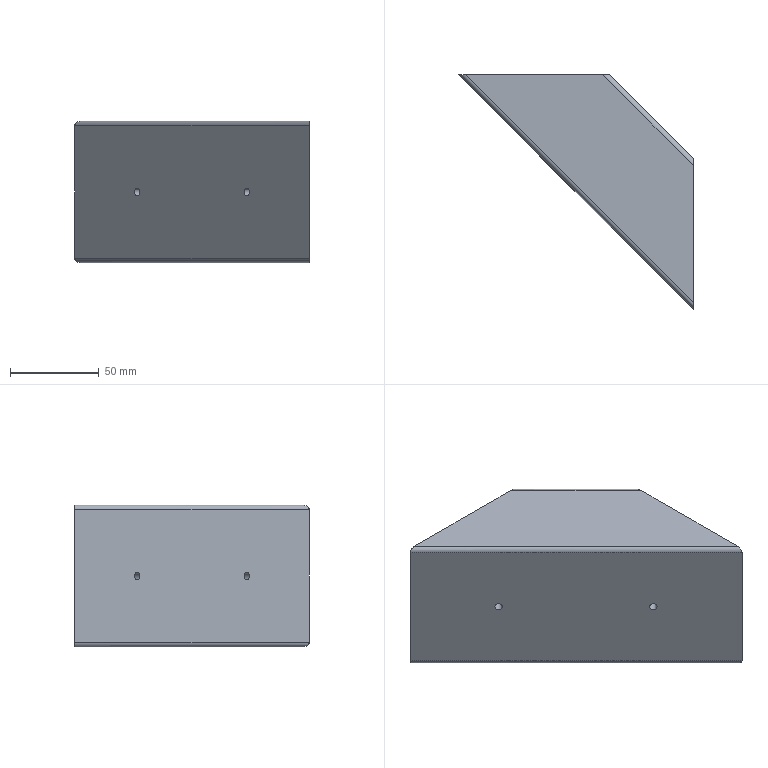Part | NX | 1 solid | 20 faces | box 132.426 x 132.426 x 80 mm | volume 195335 mm3 | plane 10 | cylinder 10 | commonest cylinder face diameters 5.236 x8 4.2 x2
STEP:
#1=CARTESIAN_POINT('',(-86.059,505.,-31.382));
#2=VERTEX_POINT('',#1);
#3=CARTESIAN_POINT('',(-89.761,505.,-34.));
#4=VERTEX_POINT('',#3);
#5=CARTESIAN_POINT('',(-89.761,505.,-31.382));
#6=DIRECTION('',(0.,1.,0.));
#7=DIRECTION('',(-1.,0.,0.));
#8=AXIS2_PLACEMENT_3D('',#5,#6,#7);
#9=ELLIPSE('',#8,3.702,2.618);
#10=EDGE_CURVE('',#2,#4,#9,.T.);
#11=ORIENTED_EDGE('',*,*,#10,.F.);
#12=CARTESIAN_POINT('',(-86.059,505.,31.382));
#13=VERTEX_POINT('',#12);
#14=CARTESIAN_POINT('',(-86.059,505.,31.382));
#15=DIRECTION('',(0.,0.,-1.));
#16=VECTOR('',#15,1000.);
#17=LINE('',#14,#16);
#18=EDGE_CURVE('',#13,#2,#17,.T.);
#19=ORIENTED_EDGE('',*,*,#18,.F.);
#20=CARTESIAN_POINT('',(-89.761,505.,34.));
#21=VERTEX_POINT('',#20);
#22=CARTESIAN_POINT('',(-89.761,505.,31.382));
#23=DIRECTION('',(0.,1.,0.));
#24=DIRECTION('',(-1.,0.,0.));
#25=AXIS2_PLACEMENT_3D('',#22,#23,#24);
#26=ELLIPSE('',#25,3.702,2.618);
#27=EDGE_CURVE('',#21,#13,#26,.T.);
#28=ORIENTED_EDGE('',*,*,#27,.F.);
#29=CARTESIAN_POINT('',(-150.239,505.,34.));
#30=VERTEX_POINT('',#29);
#31=CARTESIAN_POINT('',(-15.119,505.,34.));
#32=DIRECTION('',(1.,0.,0.));
#33=VECTOR('',#32,1000.);
#34=LINE('',#31,#33);
#35=EDGE_CURVE('',#30,#21,#34,.T.);
#36=ORIENTED_EDGE('',*,*,#35,.F.);
#37=CARTESIAN_POINT('',(-153.941,505.,31.382));
#38=VERTEX_POINT('',#37);
#39=CARTESIAN_POINT('',(-150.239,505.,31.382));
#40=DIRECTION('',(0.,1.,0.));
#41=DIRECTION('',(-1.,0.,0.));
#42=AXIS2_PLACEMENT_3D('',#39,#40,#41);
#43=ELLIPSE('',#42,3.702,2.618);
#44=EDGE_CURVE('',#38,#30,#43,.T.);
#45=ORIENTED_EDGE('',*,*,#44,.F.);
#46=CARTESIAN_POINT('',(-153.941,505.,-31.382));
#47=VERTEX_POINT('',#46);
#48=CARTESIAN_POINT('',(-153.941,505.,31.382));
#49=DIRECTION('',(0.,0.,1.));
#50=VECTOR('',#49,1000.);
#51=LINE('',#48,#50);
#52=EDGE_CURVE('',#47,#38,#51,.T.);
#53=ORIENTED_EDGE('',*,*,#52,.F.);
#54=CARTESIAN_POINT('',(-150.239,505.,-34.));
#55=VERTEX_POINT('',#54);
#56=CARTESIAN_POINT('',(-150.239,505.,-31.382));
#57=DIRECTION('',(0.,1.,0.));
#58=DIRECTION('',(-1.,0.,0.));
#59=AXIS2_PLACEMENT_3D('',#56,#57,#58);
#60=ELLIPSE('',#59,3.702,2.618);
#61=EDGE_CURVE('',#55,#47,#60,.T.);
#62=ORIENTED_EDGE('',*,*,#61,.F.);
#63=CARTESIAN_POINT('',(-15.119,505.,-34.));
#64=DIRECTION('',(-1.,0.,0.));
#65=VECTOR('',#64,1000.);
#66=LINE('',#63,#65);
#67=EDGE_CURVE('',#4,#55,#66,.T.);
#68=ORIENTED_EDGE('',*,*,#67,.F.);
#69=EDGE_LOOP('',(#11,#19,#28,#36,#45,#53,#62,#68));
#70=FACE_BOUND('',#69,.T.);
#71=CARTESIAN_POINT('',(-158.724,505.,-40.));
#72=VERTEX_POINT('',#71);
#73=CARTESIAN_POINT('',(-162.426,505.,-37.382));
#74=VERTEX_POINT('',#73);
#75=CARTESIAN_POINT('',(-158.724,505.,-37.382));
#76=DIRECTION('',(0.,1.,0.));
#77=DIRECTION('',(-1.,0.,0.));
#78=AXIS2_PLACEMENT_3D('',#75,#76,#77);
#79=ELLIPSE('',#78,3.702,2.618);
#80=EDGE_CURVE('',#72,#74,#79,.T.);
#81=ORIENTED_EDGE('',*,*,#80,.T.);
#82=CARTESIAN_POINT('',(-162.426,505.,37.382));
#83=VERTEX_POINT('',#82);
#84=CARTESIAN_POINT('',(-162.426,505.,37.382));
#85=DIRECTION('',(0.,0.,1.));
#86=VECTOR('',#85,1000.);
#87=LINE('',#84,#86);
#88=EDGE_CURVE('',#74,#83,#87,.T.);
#89=ORIENTED_EDGE('',*,*,#88,.T.);
#90=CARTESIAN_POINT('',(-158.724,505.,40.));
#91=VERTEX_POINT('',#90);
#92=CARTESIAN_POINT('',(-158.724,505.,37.382));
#93=DIRECTION('',(0.,1.,0.));
#94=DIRECTION('',(-1.,0.,0.));
#95=AXIS2_PLACEMENT_3D('',#92,#93,#94);
#96=ELLIPSE('',#95,3.702,2.618);
#97=EDGE_CURVE('',#83,#91,#96,.T.);
#98=ORIENTED_EDGE('',*,*,#97,.T.);
#99=CARTESIAN_POINT('',(-81.276,505.,40.));
#100=VERTEX_POINT('',#99);
#101=CARTESIAN_POINT('',(1126.,505.,40.));
#102=DIRECTION('',(-1.,0.,0.));
#103=VECTOR('',#102,1000.);
#104=LINE('',#101,#103);
#105=EDGE_CURVE('',#100,#91,#104,.T.);
#106=ORIENTED_EDGE('',*,*,#105,.F.);
#107=CARTESIAN_POINT('',(-77.574,505.,37.382));
#108=VERTEX_POINT('',#107);
#109=CARTESIAN_POINT('',(-81.276,505.,37.382));
#110=DIRECTION('',(0.,1.,0.));
#111=DIRECTION('',(-1.,0.,0.));
#112=AXIS2_PLACEMENT_3D('',#109,#110,#111);
#113=ELLIPSE('',#112,3.702,2.618);
#114=EDGE_CURVE('',#100,#108,#113,.T.);
#115=ORIENTED_EDGE('',*,*,#114,.T.);
#116=CARTESIAN_POINT('',(-77.574,505.,-37.382));
#117=VERTEX_POINT('',#116);
#118=CARTESIAN_POINT('',(-77.574,505.,37.382));
#119=DIRECTION('',(0.,0.,-1.));
#120=VECTOR('',#119,1000.);
#121=LINE('',#118,#120);
#122=EDGE_CURVE('',#108,#117,#121,.T.);
#123=ORIENTED_EDGE('',*,*,#122,.T.);
#124=CARTESIAN_POINT('',(-81.276,505.,-40.));
#125=VERTEX_POINT('',#124);
#126=CARTESIAN_POINT('',(-81.276,505.,-37.382));
#127=DIRECTION('',(0.,1.,0.));
#128=DIRECTION('',(-1.,0.,0.));
#129=AXIS2_PLACEMENT_3D('',#126,#127,#128);
#130=ELLIPSE('',#129,3.702,2.618);
#131=EDGE_CURVE('',#117,#125,#130,.T.);
#132=ORIENTED_EDGE('',*,*,#131,.T.);
#133=CARTESIAN_POINT('',(1126.,505.,-40.));
#134=DIRECTION('',(-1.,0.,0.));
#135=VECTOR('',#134,1000.);
#136=LINE('',#133,#135);
#137=EDGE_CURVE('',#125,#72,#136,.T.);
#138=ORIENTED_EDGE('',*,*,#137,.T.);
#139=EDGE_LOOP('',(#81,#89,#98,#106,#115,#123,#132,#138));
#140=FACE_BOUND('',#139,.T.);
#141=CARTESIAN_POINT('',(1126.,505.,37.382));
#142=DIRECTION('',(0.,1.,0.));
#143=DIRECTION('',(0.,0.,1.));
#144=AXIS2_PLACEMENT_3D('',#141,#142,#143);
#145=PLANE('',#144);
#146=ADVANCED_FACE('',(#70,#140),#145,.T.);
#147=ORIENTED_EDGE('',*,*,#114,.F.);
#148=CARTESIAN_POINT('',(-30.,453.724,40.));
#149=VERTEX_POINT('',#148);
#150=CARTESIAN_POINT('',(19.362,404.362,40.));
#151=DIRECTION('',(-0.7071,0.7071,0.));
#152=VECTOR('',#151,1000.);
#153=LINE('',#150,#152);
#154=EDGE_CURVE('',#149,#100,#153,.T.);
#155=ORIENTED_EDGE('',*,*,#154,.F.);
#156=CARTESIAN_POINT('',(-30.,457.426,37.382));
#157=VERTEX_POINT('',#156);
#158=CARTESIAN_POINT('',(-30.,453.724,37.382));
#159=DIRECTION('',(1.,0.,0.));
#160=DIRECTION('',(0.,1.,0.));
#161=AXIS2_PLACEMENT_3D('',#158,#159,#160);
#162=ELLIPSE('',#161,3.702,2.618);
#163=EDGE_CURVE('',#157,#149,#162,.T.);
#164=ORIENTED_EDGE('',*,*,#163,.F.);
#165=CARTESIAN_POINT('',(21.213,406.213,37.382));
#166=DIRECTION('',(-0.7071,0.7071,0.));
#167=VECTOR('',#166,1000.);
#168=LINE('',#165,#167);
#169=EDGE_CURVE('',#157,#108,#168,.T.);
#170=ORIENTED_EDGE('',*,*,#169,.T.);
#171=EDGE_LOOP('',(#147,#155,#164,#170));
#172=FACE_BOUND('',#171,.T.);
#173=CARTESIAN_POINT('',(19.362,404.362,37.382));
#174=DIRECTION('',(-0.7071,0.7071,0.));
#175=DIRECTION('',(-0.7071,-0.7071,0.));
#176=AXIS2_PLACEMENT_3D('',#173,#174,#175);
#177=CYLINDRICAL_SURFACE('',#176,2.618);
#178=ADVANCED_FACE('',(#172),#177,.T.);
#179=ORIENTED_EDGE('',*,*,#105,.T.);
#180=CARTESIAN_POINT('',(-30.,376.276,40.));
#181=VERTEX_POINT('',#180);
#182=CARTESIAN_POINT('',(-19.362,365.638,40.));
#183=DIRECTION('',(-0.7071,0.7071,0.));
#184=VECTOR('',#183,1000.);
#185=LINE('',#182,#184);
#186=EDGE_CURVE('',#181,#91,#185,.T.);
#187=ORIENTED_EDGE('',*,*,#186,.F.);
#188=CARTESIAN_POINT('',(-30.,535.,40.));
#189=DIRECTION('',(0.,-1.,0.));
#190=VECTOR('',#189,1000.);
#191=LINE('',#188,#190);
#192=EDGE_CURVE('',#149,#181,#191,.T.);
#193=ORIENTED_EDGE('',*,*,#192,.F.);
#194=ORIENTED_EDGE('',*,*,#154,.T.);
#195=EDGE_LOOP('',(#179,#187,#193,#194));
#196=FACE_BOUND('',#195,.T.);
#197=CARTESIAN_POINT('',(-19.362,365.638,40.));
#198=DIRECTION('',(0.,0.,-1.));
#199=DIRECTION('',(-1.,0.,0.));
#200=AXIS2_PLACEMENT_3D('',#197,#198,#199);
#201=PLANE('',#200);
#202=ADVANCED_FACE('',(#196),#201,.F.);
#203=ORIENTED_EDGE('',*,*,#97,.F.);
#204=CARTESIAN_POINT('',(-30.,372.574,37.382));
#205=VERTEX_POINT('',#204);
#206=CARTESIAN_POINT('',(-21.213,363.787,37.382));
#207=DIRECTION('',(-0.7071,0.7071,0.));
#208=VECTOR('',#207,1000.);
#209=LINE('',#206,#208);
#210=EDGE_CURVE('',#205,#83,#209,.T.);
#211=ORIENTED_EDGE('',*,*,#210,.F.);
#212=CARTESIAN_POINT('',(-30.,376.276,37.382));
#213=DIRECTION('',(1.,0.,0.));
#214=DIRECTION('',(0.,1.,0.));
#215=AXIS2_PLACEMENT_3D('',#212,#213,#214);
#216=ELLIPSE('',#215,3.702,2.618);
#217=EDGE_CURVE('',#181,#205,#216,.T.);
#218=ORIENTED_EDGE('',*,*,#217,.F.);
#219=ORIENTED_EDGE('',*,*,#186,.T.);
#220=EDGE_LOOP('',(#203,#211,#218,#219));
#221=FACE_BOUND('',#220,.T.);
#222=CARTESIAN_POINT('',(-19.362,365.638,37.382));
#223=DIRECTION('',(-0.7071,0.7071,0.));
#224=DIRECTION('',(-0.7071,-0.7071,0.));
#225=AXIS2_PLACEMENT_3D('',#222,#223,#224);
#226=CYLINDRICAL_SURFACE('',#225,2.618);
#227=ADVANCED_FACE('',(#221),#226,.T.);
#228=CARTESIAN_POINT('',(-66.84,409.414,0.));
#229=VERTEX_POINT('',#228);
#230=CARTESIAN_POINT('',(-65.355,407.929,0.));
#231=DIRECTION('',(-0.7071,-0.7071,0.));
#232=DIRECTION('',(-0.7071,0.7071,0.));
#233=AXIS2_PLACEMENT_3D('',#230,#231,#232);
#234=CIRCLE('',#233,2.1);
#235=EDGE_CURVE('',#229,#229,#234,.T.);
#236=ORIENTED_EDGE('',*,*,#235,.F.);
#237=EDGE_LOOP('',(#236));
#238=FACE_BOUND('',#237,.T.);
#239=CARTESIAN_POINT('',(-128.556,471.13,0.));
#240=VERTEX_POINT('',#239);
#241=CARTESIAN_POINT('',(-127.071,469.645,0.));
#242=DIRECTION('',(-0.7071,-0.7071,0.));
#243=DIRECTION('',(-0.7071,0.7071,0.));
#244=AXIS2_PLACEMENT_3D('',#241,#242,#243);
#245=CIRCLE('',#244,2.1);
#246=EDGE_CURVE('',#240,#240,#245,.T.);
#247=ORIENTED_EDGE('',*,*,#246,.F.);
#248=EDGE_LOOP('',(#247));
#249=FACE_BOUND('',#248,.T.);
#250=ORIENTED_EDGE('',*,*,#88,.F.);
#251=CARTESIAN_POINT('',(-30.,372.574,-37.382));
#252=VERTEX_POINT('',#251);
#253=CARTESIAN_POINT('',(-21.213,363.787,-37.382));
#254=DIRECTION('',(-0.7071,0.7071,0.));
#255=VECTOR('',#254,1000.);
#256=LINE('',#253,#255);
#257=EDGE_CURVE('',#252,#74,#256,.T.);
#258=ORIENTED_EDGE('',*,*,#257,.F.);
#259=CARTESIAN_POINT('',(-30.,372.574,37.382));
#260=DIRECTION('',(0.,0.,-1.));
#261=VECTOR('',#260,1000.);
#262=LINE('',#259,#261);
#263=EDGE_CURVE('',#205,#252,#262,.T.);
#264=ORIENTED_EDGE('',*,*,#263,.F.);
#265=ORIENTED_EDGE('',*,*,#210,.T.);
#266=EDGE_LOOP('',(#250,#258,#264,#265));
#267=FACE_BOUND('',#266,.T.);
#268=CARTESIAN_POINT('',(-21.213,363.787,37.382));
#269=DIRECTION('',(0.7071,0.7071,0.));
#270=DIRECTION('',(-0.7071,0.7071,0.));
#271=AXIS2_PLACEMENT_3D('',#268,#269,#270);
#272=PLANE('',#271);
#273=ADVANCED_FACE('',(#238,#249,#267),#272,.F.);
#274=ORIENTED_EDGE('',*,*,#80,.F.);
#275=CARTESIAN_POINT('',(-30.,376.276,-40.));
#276=VERTEX_POINT('',#275);
#277=CARTESIAN_POINT('',(-19.362,365.638,-40.));
#278=DIRECTION('',(-0.7071,0.7071,0.));
#279=VECTOR('',#278,1000.);
#280=LINE('',#277,#279);
#281=EDGE_CURVE('',#276,#72,#280,.T.);
#282=ORIENTED_EDGE('',*,*,#281,.F.);
#283=CARTESIAN_POINT('',(-30.,376.276,-37.382));
#284=DIRECTION('',(1.,0.,0.));
#285=DIRECTION('',(0.,1.,0.));
#286=AXIS2_PLACEMENT_3D('',#283,#284,#285);
#287=ELLIPSE('',#286,3.702,2.618);
#288=EDGE_CURVE('',#252,#276,#287,.T.);
#289=ORIENTED_EDGE('',*,*,#288,.F.);
#290=ORIENTED_EDGE('',*,*,#257,.T.);
#291=EDGE_LOOP('',(#274,#282,#289,#290));
#292=FACE_BOUND('',#291,.T.);
#293=CARTESIAN_POINT('',(-19.362,365.638,-37.382));
#294=DIRECTION('',(-0.7071,0.7071,0.));
#295=DIRECTION('',(-0.7071,-0.7071,0.));
#296=AXIS2_PLACEMENT_3D('',#293,#294,#295);
#297=CYLINDRICAL_SURFACE('',#296,2.618);
#298=ADVANCED_FACE('',(#292),#297,.T.);
#299=ORIENTED_EDGE('',*,*,#137,.F.);
#300=CARTESIAN_POINT('',(-30.,453.724,-40.));
#301=VERTEX_POINT('',#300);
#302=CARTESIAN_POINT('',(19.362,404.362,-40.));
#303=DIRECTION('',(-0.7071,0.7071,0.));
#304=VECTOR('',#303,1000.);
#305=LINE('',#302,#304);
#306=EDGE_CURVE('',#301,#125,#305,.T.);
#307=ORIENTED_EDGE('',*,*,#306,.F.);
#308=CARTESIAN_POINT('',(-30.,535.,-40.));
#309=DIRECTION('',(0.,-1.,0.));
#310=VECTOR('',#309,1000.);
#311=LINE('',#308,#310);
#312=EDGE_CURVE('',#301,#276,#311,.T.);
#313=ORIENTED_EDGE('',*,*,#312,.T.);
#314=ORIENTED_EDGE('',*,*,#281,.T.);
#315=EDGE_LOOP('',(#299,#307,#313,#314));
#316=FACE_BOUND('',#315,.T.);
#317=CARTESIAN_POINT('',(-19.362,365.638,-40.));
#318=DIRECTION('',(0.,0.,1.));
#319=DIRECTION('',(1.,0.,0.));
#320=AXIS2_PLACEMENT_3D('',#317,#318,#319);
#321=PLANE('',#320);
#322=ADVANCED_FACE('',(#316),#321,.F.);
#323=ORIENTED_EDGE('',*,*,#131,.F.);
#324=CARTESIAN_POINT('',(-30.,457.426,-37.382));
#325=VERTEX_POINT('',#324);
#326=CARTESIAN_POINT('',(21.213,406.213,-37.382));
#327=DIRECTION('',(-0.7071,0.7071,0.));
#328=VECTOR('',#327,1000.);
#329=LINE('',#326,#328);
#330=EDGE_CURVE('',#325,#117,#329,.T.);
#331=ORIENTED_EDGE('',*,*,#330,.F.);
#332=CARTESIAN_POINT('',(-30.,453.724,-37.382));
#333=DIRECTION('',(1.,0.,0.));
#334=DIRECTION('',(0.,1.,0.));
#335=AXIS2_PLACEMENT_3D('',#332,#333,#334);
#336=ELLIPSE('',#335,3.702,2.618);
#337=EDGE_CURVE('',#301,#325,#336,.T.);
#338=ORIENTED_EDGE('',*,*,#337,.F.);
#339=ORIENTED_EDGE('',*,*,#306,.T.);
#340=EDGE_LOOP('',(#323,#331,#338,#339));
#341=FACE_BOUND('',#340,.T.);
#342=CARTESIAN_POINT('',(19.362,404.362,-37.382));
#343=DIRECTION('',(-0.7071,0.7071,0.));
#344=DIRECTION('',(-0.7071,-0.7071,0.));
#345=AXIS2_PLACEMENT_3D('',#342,#343,#344);
#346=CYLINDRICAL_SURFACE('',#345,2.618);
#347=ADVANCED_FACE('',(#341),#346,.T.);
#348=ORIENTED_EDGE('',*,*,#122,.F.);
#349=ORIENTED_EDGE('',*,*,#169,.F.);
#350=CARTESIAN_POINT('',(-30.,457.426,37.382));
#351=DIRECTION('',(0.,0.,1.));
#352=VECTOR('',#351,1000.);
#353=LINE('',#350,#352);
#354=EDGE_CURVE('',#325,#157,#353,.T.);
#355=ORIENTED_EDGE('',*,*,#354,.F.);
#356=ORIENTED_EDGE('',*,*,#330,.T.);
#357=EDGE_LOOP('',(#348,#349,#355,#356));
#358=FACE_BOUND('',#357,.T.);
#359=CARTESIAN_POINT('',(21.213,406.213,37.382));
#360=DIRECTION('',(-0.7071,-0.7071,0.));
#361=DIRECTION('',(0.7071,-0.7071,0.));
#362=AXIS2_PLACEMENT_3D('',#359,#360,#361);
#363=PLANE('',#362);
#364=ADVANCED_FACE('',(#358),#363,.F.);
#365=CARTESIAN_POINT('',(-30.,381.059,31.382));
#366=VERTEX_POINT('',#365);
#367=CARTESIAN_POINT('',(-30.,381.059,-31.382));
#368=VERTEX_POINT('',#367);
#369=CARTESIAN_POINT('',(-30.,381.059,31.382));
#370=DIRECTION('',(0.,0.,-1.));
#371=VECTOR('',#370,1000.);
#372=LINE('',#369,#371);
#373=EDGE_CURVE('',#366,#368,#372,.T.);
#374=ORIENTED_EDGE('',*,*,#373,.F.);
#375=CARTESIAN_POINT('',(-30.,384.761,34.));
#376=VERTEX_POINT('',#375);
#377=CARTESIAN_POINT('',(-30.,384.761,31.382));
#378=DIRECTION('',(1.,0.,0.));
#379=DIRECTION('',(0.,1.,0.));
#380=AXIS2_PLACEMENT_3D('',#377,#378,#379);
#381=ELLIPSE('',#380,3.702,2.618);
#382=EDGE_CURVE('',#376,#366,#381,.T.);
#383=ORIENTED_EDGE('',*,*,#382,.F.);
#384=CARTESIAN_POINT('',(-30.,445.239,34.));
#385=VERTEX_POINT('',#384);
#386=CARTESIAN_POINT('',(-30.,369.881,34.));
#387=DIRECTION('',(0.,-1.,0.));
#388=VECTOR('',#387,1000.);
#389=LINE('',#386,#388);
#390=EDGE_CURVE('',#385,#376,#389,.T.);
#391=ORIENTED_EDGE('',*,*,#390,.F.);
#392=CARTESIAN_POINT('',(-30.,448.941,31.382));
#393=VERTEX_POINT('',#392);
#394=CARTESIAN_POINT('',(-30.,445.239,31.382));
#395=DIRECTION('',(1.,0.,0.));
#396=DIRECTION('',(0.,1.,0.));
#397=AXIS2_PLACEMENT_3D('',#394,#395,#396);
#398=ELLIPSE('',#397,3.702,2.618);
#399=EDGE_CURVE('',#393,#385,#398,.T.);
#400=ORIENTED_EDGE('',*,*,#399,.F.);
#401=CARTESIAN_POINT('',(-30.,448.941,-31.382));
#402=VERTEX_POINT('',#401);
#403=CARTESIAN_POINT('',(-30.,448.941,31.382));
#404=DIRECTION('',(0.,0.,1.));
#405=VECTOR('',#404,1000.);
#406=LINE('',#403,#405);
#407=EDGE_CURVE('',#402,#393,#406,.T.);
#408=ORIENTED_EDGE('',*,*,#407,.F.);
#409=CARTESIAN_POINT('',(-30.,445.239,-34.));
#410=VERTEX_POINT('',#409);
#411=CARTESIAN_POINT('',(-30.,445.239,-31.382));
#412=DIRECTION('',(1.,0.,0.));
#413=DIRECTION('',(0.,1.,0.));
#414=AXIS2_PLACEMENT_3D('',#411,#412,#413);
#415=ELLIPSE('',#414,3.702,2.618);
#416=EDGE_CURVE('',#410,#402,#415,.T.);
#417=ORIENTED_EDGE('',*,*,#416,.F.);
#418=CARTESIAN_POINT('',(-30.,384.761,-34.));
#419=VERTEX_POINT('',#418);
#420=CARTESIAN_POINT('',(-30.,369.881,-34.));
#421=DIRECTION('',(0.,1.,0.));
#422=VECTOR('',#421,1000.);
#423=LINE('',#420,#422);
#424=EDGE_CURVE('',#419,#410,#423,.T.);
#425=ORIENTED_EDGE('',*,*,#424,.F.);
#426=CARTESIAN_POINT('',(-30.,384.761,-31.382));
#427=DIRECTION('',(1.,0.,0.));
#428=DIRECTION('',(0.,1.,0.));
#429=AXIS2_PLACEMENT_3D('',#426,#427,#428);
#430=ELLIPSE('',#429,3.702,2.618);
#431=EDGE_CURVE('',#368,#419,#430,.T.);
#432=ORIENTED_EDGE('',*,*,#431,.F.);
#433=EDGE_LOOP('',(#374,#383,#391,#400,#408,#417,#425,#432));
#434=FACE_BOUND('',#433,.T.);
#435=ORIENTED_EDGE('',*,*,#217,.T.);
#436=ORIENTED_EDGE('',*,*,#263,.T.);
#437=ORIENTED_EDGE('',*,*,#288,.T.);
#438=ORIENTED_EDGE('',*,*,#312,.F.);
#439=ORIENTED_EDGE('',*,*,#337,.T.);
#440=ORIENTED_EDGE('',*,*,#354,.T.);
#441=ORIENTED_EDGE('',*,*,#163,.T.);
#442=ORIENTED_EDGE('',*,*,#192,.T.);
#443=EDGE_LOOP('',(#435,#436,#437,#438,#439,#440,#441,#442));
#444=FACE_BOUND('',#443,.T.);
#445=CARTESIAN_POINT('',(-30.,535.,-37.382));
#446=DIRECTION('',(1.,0.,0.));
#447=DIRECTION('',(0.,0.,-1.));
#448=AXIS2_PLACEMENT_3D('',#445,#446,#447);
#449=PLANE('',#448);
#450=ADVANCED_FACE('',(#434,#444),#449,.T.);
#451=CARTESIAN_POINT('',(-15.119,369.881,-34.));
#452=DIRECTION('',(-0.7071,0.7071,0.));
#453=VECTOR('',#452,1000.);
#454=LINE('',#451,#453);
#455=EDGE_CURVE('',#419,#55,#454,.T.);
#456=ORIENTED_EDGE('',*,*,#455,.T.);
#457=ORIENTED_EDGE('',*,*,#61,.T.);
#458=CARTESIAN_POINT('',(-16.971,368.029,-31.382));
#459=DIRECTION('',(-0.7071,0.7071,0.));
#460=VECTOR('',#459,1000.);
#461=LINE('',#458,#460);
#462=EDGE_CURVE('',#368,#47,#461,.T.);
#463=ORIENTED_EDGE('',*,*,#462,.F.);
#464=ORIENTED_EDGE('',*,*,#431,.T.);
#465=EDGE_LOOP('',(#456,#457,#463,#464));
#466=FACE_BOUND('',#465,.T.);
#467=CARTESIAN_POINT('',(-15.119,369.881,-31.382));
#468=DIRECTION('',(-0.7071,0.7071,0.));
#469=DIRECTION('',(-0.7071,-0.7071,0.));
#470=AXIS2_PLACEMENT_3D('',#467,#468,#469);
#471=CYLINDRICAL_SURFACE('',#470,2.618);
#472=ADVANCED_FACE('',(#466),#471,.F.);
#473=CARTESIAN_POINT('',(-62.598,413.656,0.));
#474=VERTEX_POINT('',#473);
#475=CARTESIAN_POINT('',(-61.113,412.172,0.));
#476=DIRECTION('',(0.7071,0.7071,0.));
#477=DIRECTION('',(-0.7071,0.7071,0.));
#478=AXIS2_PLACEMENT_3D('',#475,#476,#477);
#479=CIRCLE('',#478,2.1);
#480=EDGE_CURVE('',#474,#474,#479,.T.);
#481=ORIENTED_EDGE('',*,*,#480,.F.);
#482=EDGE_LOOP('',(#481));
#483=FACE_BOUND('',#482,.T.);
#484=CARTESIAN_POINT('',(-124.313,475.372,0.));
#485=VERTEX_POINT('',#484);
#486=CARTESIAN_POINT('',(-122.828,473.887,0.));
#487=DIRECTION('',(0.7071,0.7071,0.));
#488=DIRECTION('',(-0.7071,0.7071,0.));
#489=AXIS2_PLACEMENT_3D('',#486,#487,#488);
#490=CIRCLE('',#489,2.1);
#491=EDGE_CURVE('',#485,#485,#490,.T.);
#492=ORIENTED_EDGE('',*,*,#491,.F.);
#493=EDGE_LOOP('',(#492));
#494=FACE_BOUND('',#493,.T.);
#495=ORIENTED_EDGE('',*,*,#462,.T.);
#496=ORIENTED_EDGE('',*,*,#52,.T.);
#497=CARTESIAN_POINT('',(-16.971,368.029,31.382));
#498=DIRECTION('',(-0.7071,0.7071,0.));
#499=VECTOR('',#498,1000.);
#500=LINE('',#497,#499);
#501=EDGE_CURVE('',#366,#38,#500,.T.);
#502=ORIENTED_EDGE('',*,*,#501,.F.);
#503=ORIENTED_EDGE('',*,*,#373,.T.);
#504=EDGE_LOOP('',(#495,#496,#502,#503));
#505=FACE_BOUND('',#504,.T.);
#506=CARTESIAN_POINT('',(-16.971,368.029,31.382));
#507=DIRECTION('',(0.7071,0.7071,0.));
#508=DIRECTION('',(-0.7071,0.7071,0.));
#509=AXIS2_PLACEMENT_3D('',#506,#507,#508);
#510=PLANE('',#509);
#511=ADVANCED_FACE('',(#483,#494,#505),#510,.T.);
#512=ORIENTED_EDGE('',*,*,#501,.T.);
#513=ORIENTED_EDGE('',*,*,#44,.T.);
#514=CARTESIAN_POINT('',(-15.119,369.881,34.));
#515=DIRECTION('',(-0.7071,0.7071,0.));
#516=VECTOR('',#515,1000.);
#517=LINE('',#514,#516);
#518=EDGE_CURVE('',#376,#30,#517,.T.);
#519=ORIENTED_EDGE('',*,*,#518,.F.);
#520=ORIENTED_EDGE('',*,*,#382,.T.);
#521=EDGE_LOOP('',(#512,#513,#519,#520));
#522=FACE_BOUND('',#521,.T.);
#523=CARTESIAN_POINT('',(-15.119,369.881,31.382));
#524=DIRECTION('',(-0.7071,0.7071,0.));
#525=DIRECTION('',(-0.7071,-0.7071,0.));
#526=AXIS2_PLACEMENT_3D('',#523,#524,#525);
#527=CYLINDRICAL_SURFACE('',#526,2.618);
#528=ADVANCED_FACE('',(#522),#527,.F.);
#529=ORIENTED_EDGE('',*,*,#518,.T.);
#530=ORIENTED_EDGE('',*,*,#35,.T.);
#531=CARTESIAN_POINT('',(15.119,400.119,34.));
#532=DIRECTION('',(-0.7071,0.7071,0.));
#533=VECTOR('',#532,1000.);
#534=LINE('',#531,#533);
#535=EDGE_CURVE('',#385,#21,#534,.T.);
#536=ORIENTED_EDGE('',*,*,#535,.F.);
#537=ORIENTED_EDGE('',*,*,#390,.T.);
#538=EDGE_LOOP('',(#529,#530,#536,#537));
#539=FACE_BOUND('',#538,.T.);
#540=CARTESIAN_POINT('',(-15.119,369.881,34.));
#541=DIRECTION('',(0.,0.,-1.));
#542=DIRECTION('',(-1.,0.,0.));
#543=AXIS2_PLACEMENT_3D('',#540,#541,#542);
#544=PLANE('',#543);
#545=ADVANCED_FACE('',(#539),#544,.T.);
#546=ORIENTED_EDGE('',*,*,#535,.T.);
#547=ORIENTED_EDGE('',*,*,#27,.T.);
#548=CARTESIAN_POINT('',(16.971,401.971,31.382));
#549=DIRECTION('',(-0.7071,0.7071,0.));
#550=VECTOR('',#549,1000.);
#551=LINE('',#548,#550);
#552=EDGE_CURVE('',#393,#13,#551,.T.);
#553=ORIENTED_EDGE('',*,*,#552,.F.);
#554=ORIENTED_EDGE('',*,*,#399,.T.);
#555=EDGE_LOOP('',(#546,#547,#553,#554));
#556=FACE_BOUND('',#555,.T.);
#557=CARTESIAN_POINT('',(15.119,400.119,31.382));
#558=DIRECTION('',(-0.7071,0.7071,0.));
#559=DIRECTION('',(-0.7071,-0.7071,0.));
#560=AXIS2_PLACEMENT_3D('',#557,#558,#559);
#561=CYLINDRICAL_SURFACE('',#560,2.618);
#562=ADVANCED_FACE('',(#556),#561,.F.);
#563=ORIENTED_EDGE('',*,*,#552,.T.);
#564=ORIENTED_EDGE('',*,*,#18,.T.);
#565=CARTESIAN_POINT('',(16.971,401.971,-31.382));
#566=DIRECTION('',(-0.7071,0.7071,0.));
#567=VECTOR('',#566,1000.);
#568=LINE('',#565,#567);
#569=EDGE_CURVE('',#402,#2,#568,.T.);
#570=ORIENTED_EDGE('',*,*,#569,.F.);
#571=ORIENTED_EDGE('',*,*,#407,.T.);
#572=EDGE_LOOP('',(#563,#564,#570,#571));
#573=FACE_BOUND('',#572,.T.);
#574=CARTESIAN_POINT('',(16.971,401.971,31.382));
#575=DIRECTION('',(-0.7071,-0.7071,0.));
#576=DIRECTION('',(0.7071,-0.7071,0.));
#577=AXIS2_PLACEMENT_3D('',#574,#575,#576);
#578=PLANE('',#577);
#579=ADVANCED_FACE('',(#573),#578,.T.);
#580=ORIENTED_EDGE('',*,*,#569,.T.);
#581=ORIENTED_EDGE('',*,*,#10,.T.);
#582=CARTESIAN_POINT('',(15.119,400.119,-34.));
#583=DIRECTION('',(-0.7071,0.7071,0.));
#584=VECTOR('',#583,1000.);
#585=LINE('',#582,#584);
#586=EDGE_CURVE('',#410,#4,#585,.T.);
#587=ORIENTED_EDGE('',*,*,#586,.F.);
#588=ORIENTED_EDGE('',*,*,#416,.T.);
#589=EDGE_LOOP('',(#580,#581,#587,#588));
#590=FACE_BOUND('',#589,.T.);
#591=CARTESIAN_POINT('',(15.119,400.119,-31.382));
#592=DIRECTION('',(-0.7071,0.7071,0.));
#593=DIRECTION('',(-0.7071,-0.7071,0.));
#594=AXIS2_PLACEMENT_3D('',#591,#592,#593);
#595=CYLINDRICAL_SURFACE('',#594,2.618);
#596=ADVANCED_FACE('',(#590),#595,.F.);
#597=ORIENTED_EDGE('',*,*,#586,.T.);
#598=ORIENTED_EDGE('',*,*,#67,.T.);
#599=ORIENTED_EDGE('',*,*,#455,.F.);
#600=ORIENTED_EDGE('',*,*,#424,.T.);
#601=EDGE_LOOP('',(#597,#598,#599,#600));
#602=FACE_BOUND('',#601,.T.);
#603=CARTESIAN_POINT('',(-15.119,369.881,-34.));
#604=DIRECTION('',(0.,0.,1.));
#605=DIRECTION('',(1.,0.,0.));
#606=AXIS2_PLACEMENT_3D('',#603,#604,#605);
#607=PLANE('',#606);
#608=ADVANCED_FACE('',(#602),#607,.T.);
#609=ORIENTED_EDGE('',*,*,#491,.T.);
#610=EDGE_LOOP('',(#609));
#611=FACE_BOUND('',#610,.T.);
#612=ORIENTED_EDGE('',*,*,#246,.T.);
#613=EDGE_LOOP('',(#612));
#614=FACE_BOUND('',#613,.T.);
#615=CARTESIAN_POINT('',(-127.071,469.645,0.));
#616=DIRECTION('',(-0.7071,-0.7071,0.));
#617=DIRECTION('',(-0.7071,0.7071,0.));
#618=AXIS2_PLACEMENT_3D('',#615,#616,#617);
#619=CYLINDRICAL_SURFACE('',#618,2.1);
#620=ADVANCED_FACE('',(#611,#614),#619,.F.);
#621=ORIENTED_EDGE('',*,*,#480,.T.);
#622=EDGE_LOOP('',(#621));
#623=FACE_BOUND('',#622,.T.);
#624=ORIENTED_EDGE('',*,*,#235,.T.);
#625=EDGE_LOOP('',(#624));
#626=FACE_BOUND('',#625,.T.);
#627=CARTESIAN_POINT('',(-65.355,407.929,0.));
#628=DIRECTION('',(-0.7071,-0.7071,0.));
#629=DIRECTION('',(-0.7071,0.7071,0.));
#630=AXIS2_PLACEMENT_3D('',#627,#628,#629);
#631=CYLINDRICAL_SURFACE('',#630,2.1);
#632=ADVANCED_FACE('',(#623,#626),#631,.F.);
#633=CLOSED_SHELL('',(#146,#178,#202,#227,#273,#298,#322,#347,#364,#450,#472,#511,#528,#545,#562,#579,#596,#608,#620,#632));
#634=MANIFOLD_SOLID_BREP('',#633);
#635=(LENGTH_UNIT()NAMED_UNIT(*)SI_UNIT(.MILLI.,.METRE.));
#636=UNCERTAINTY_MEASURE_WITH_UNIT(LENGTH_MEASURE(0.00001),#635,'','');
#637=(NAMED_UNIT(*)PLANE_ANGLE_UNIT()SI_UNIT($,.RADIAN.));
#638=(NAMED_UNIT(*)SI_UNIT($,.STERADIAN.)SOLID_ANGLE_UNIT());
#639=(GEOMETRIC_REPRESENTATION_CONTEXT(3)GLOBAL_UNCERTAINTY_ASSIGNED_CONTEXT((#636))GLOBAL_UNIT_ASSIGNED_CONTEXT((#635,#637,#638))REPRESENTATION_CONTEXT('',''));
#640=ADVANCED_BREP_SHAPE_REPRESENTATION('',(#634),#639);